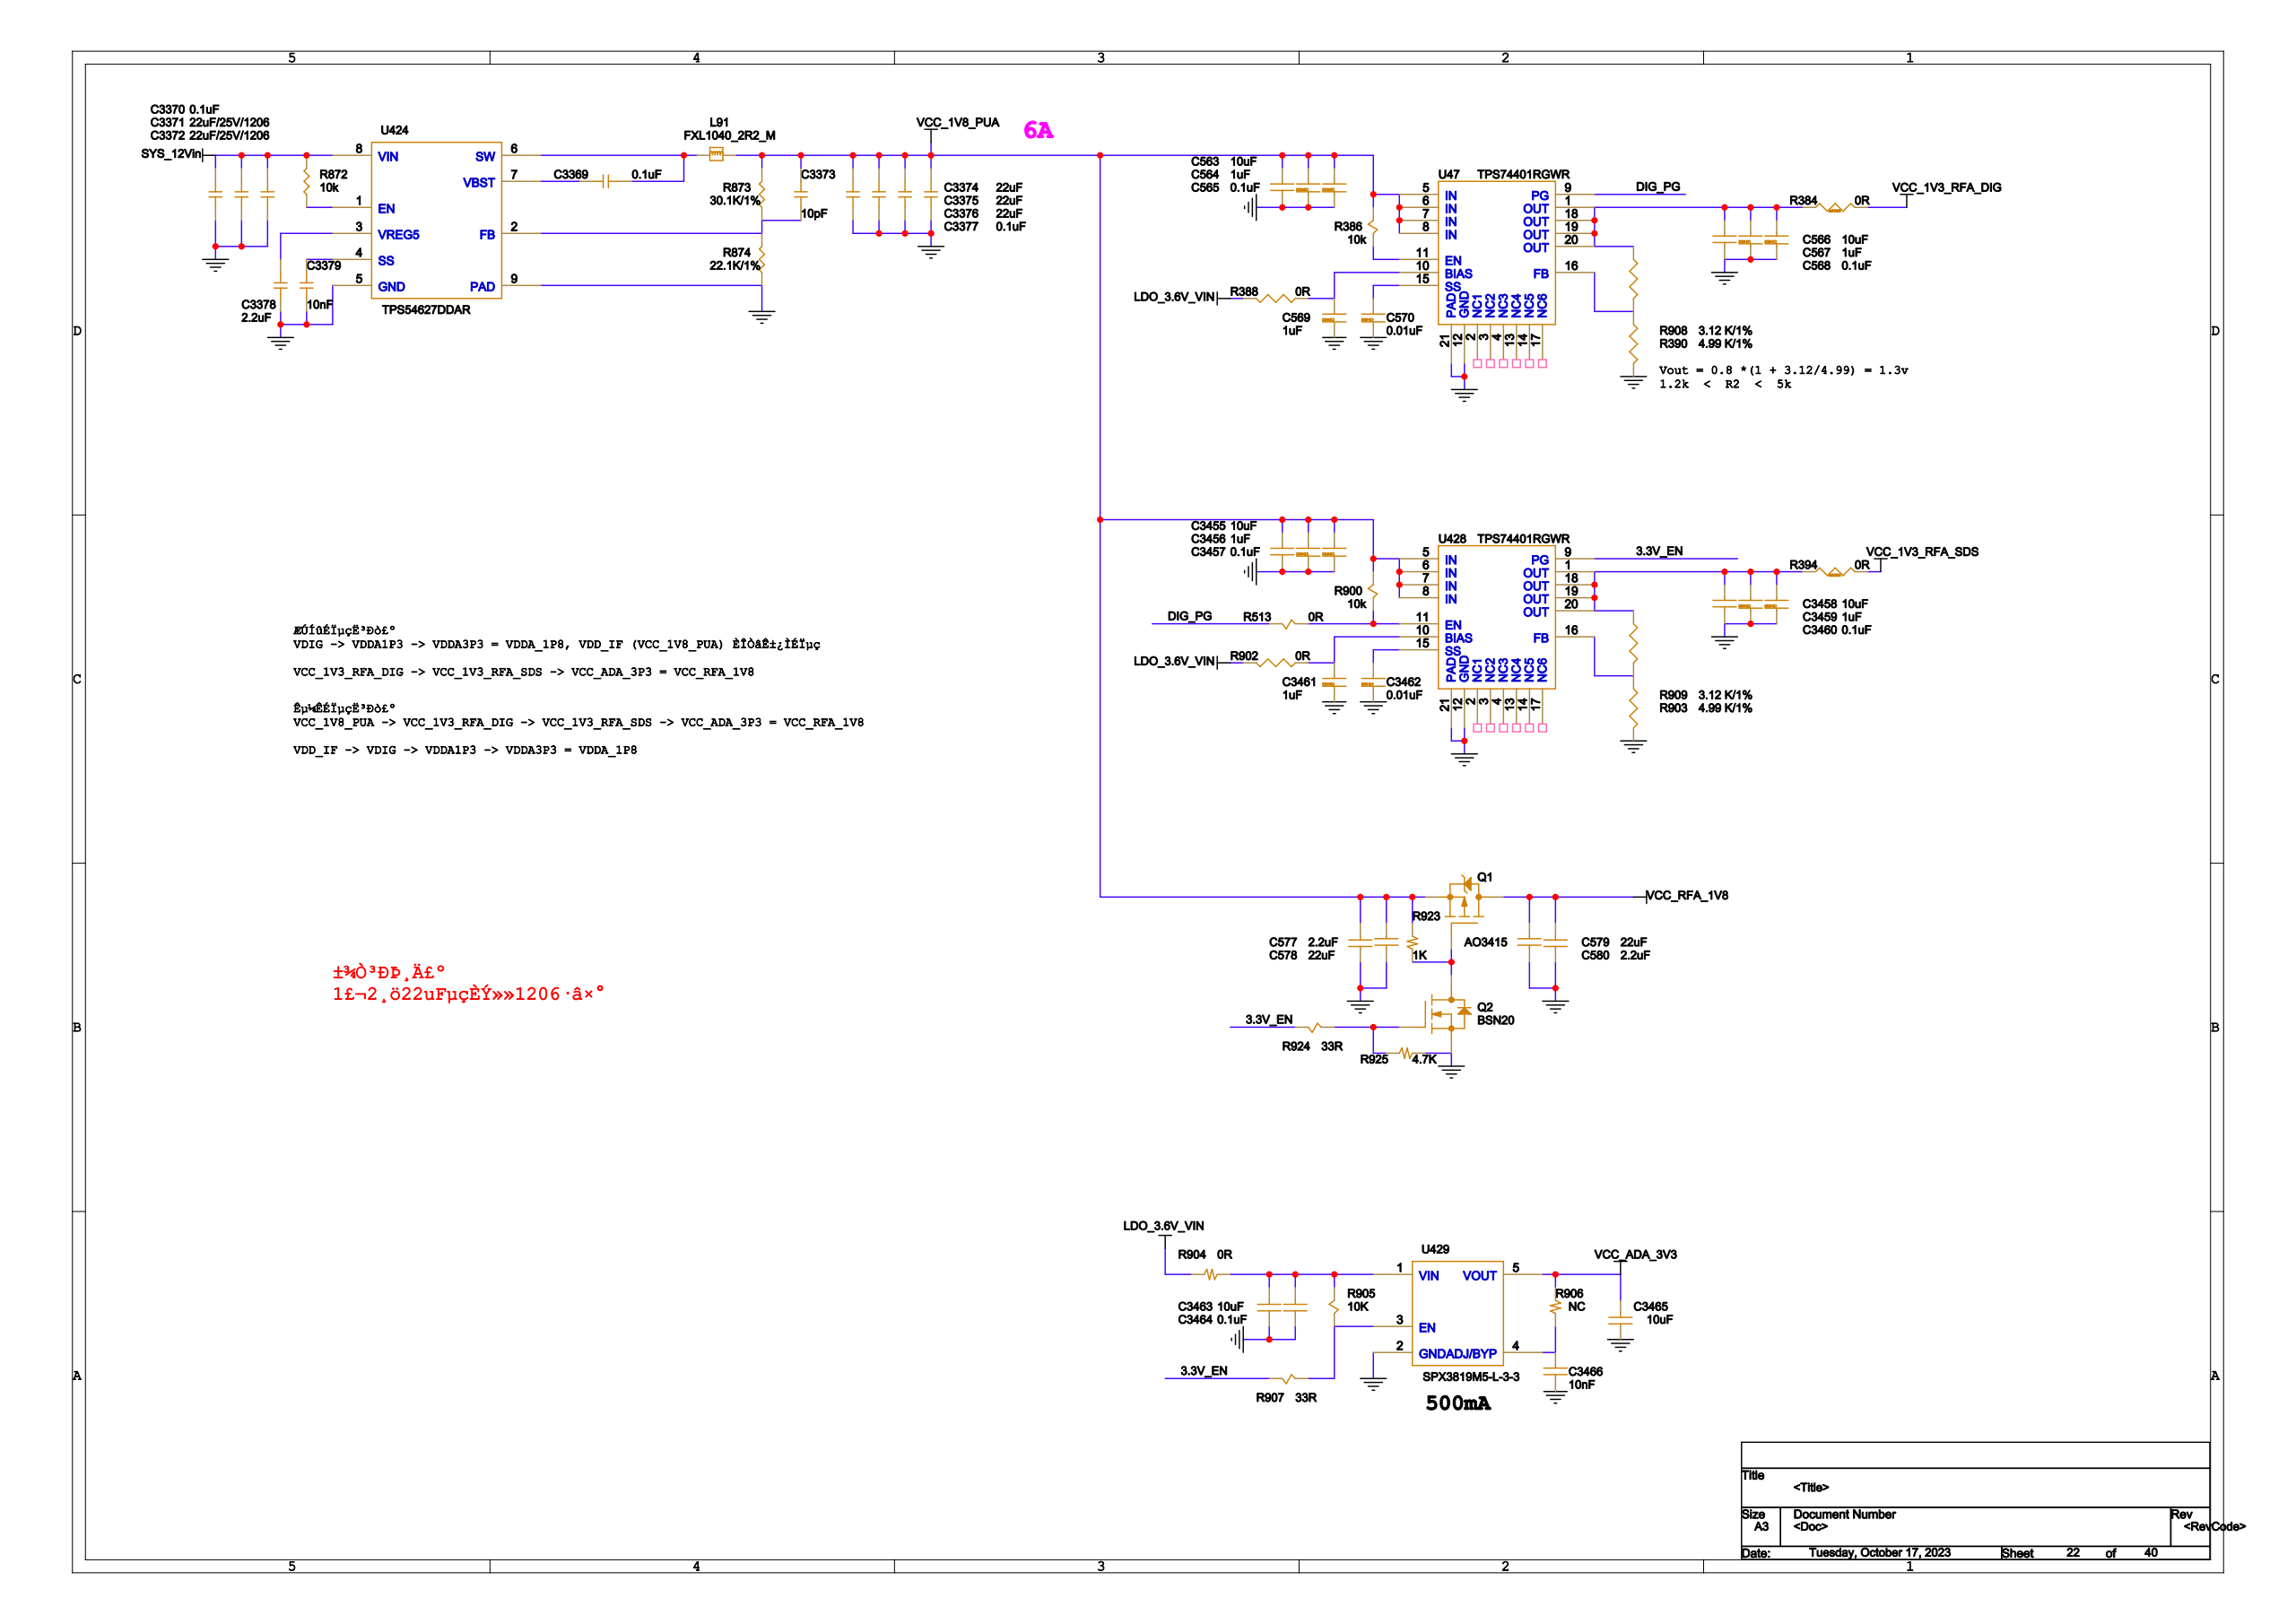Circuit board | Cadence Allegro | 1793 parts | 1223 nets | one sheet of the schematic
Parts on this sheet (reference | value | footprint):
C563 | 10uF | C0402
C564 | 1uF | C0402
C565 | 0.1uF | C0402
C566 | 10uF | C0402
C567 | 1uF | C0402
C568 | 0.1uF | C0402
C569 | 1uF | C0402
C570 | 0.01uF | C0402
C577 | 2.2uF | C0402
C578 | 22uF | C0603
C579 | 22uF | C0603
C580 | 2.2uF | C0402
C3369 | 0.1uF | C0402
C3370 | 0.1uF | C0402
C3371 | 22uF/25V/1206 | 1206
C3372 | 22uF/25V/1206 | 1206
C3373 | 10pF | C0402
C3374 | 22uF | C0603
C3375 | 22uF | C0603
C3376 | 22uF | C0603
C3377 | 0.1uF | C0402
C3378 | 2.2uF | C0402
C3379 | 10nF | C0402
C3455 | 10uF | C0402
C3456 | 1uF | C0402
C3457 | 0.1uF | C0402
C3458 | 10uF | C0402
C3459 | 1uF | C0402
C3460 | 0.1uF | C0402
C3461 | 1uF | C0402
C3462 | 0.01uF | C0402
C3463 | 10uF | C0402
C3464 | 0.1uF | C0402
C3465 | 10uF | C0402
C3466 | 10nF | C0402
L91 | FXL1040_2R2_M | SMD_11_5X10
Q1 | AO3415 | SOT23
Q2 | BSN20 | SOT23
R384 | 0R | R0805
R386 | 10K | R0402
R388 | 0R | R0402
R390 | 4.99 K/1% | R0402
R394 | 0R | R0805
R513 | 0R | R0402
R872 | 10k | R0402
R873 | 30.1K/1% | R0402
R874 | 22.1K/1% | R0402
R900 | 10K | R0402
R902 | 0R | R0402
R903 | 4.99 K/1% | R0402
R904 | 0R | R0402
R905 | 10K | R0402
R906 | NC | R0402
R907 | 33R | R0402
R908 | 3.12 K/1% | R0402
R909 | 3.12 K/1% | R0402
R923 | 1K | R0402
R924 | 33R | R0402
R925 | 4.7K | R0402
U47 | TPS74401RGWR | TPS74401RGWR_VQFN
U424 | TPS54627DDAR | POWER-SO8
U428 | TPS74401RGWR | TPS74401RGWR_VQFN
U429 | SPX3819M5-L-3-3 | SOT-23-5
Nets of these parts (net: part-pin ...):
GND: C563-2 C564-1 C565-1 C566-2 C567-1 C568-1 C569-1 C570-1 C577-1 C578-2 C579-2 C580-1 C3370-1 C3371-1 C3372-1 C3374-1 C3375-1 C3376-1 C3377-1 C3378-1 C3379-1 C3455-2 C3456-1 C3457-1 C3458-2 C3459-1 C3460-1 C3461-1 C3462-1 C3463-1 C3464-1 C3465-1 C3466-2 Q2-2 R390-2 R874-2 R903-2 R925-2 U47-12 U47-21 U424-5 U424-9 U428-12 U428-21 U429-2
SYS_12VIN: C3370-2 C3371-2 C3372-2 R872-1 U424-8
LDO_3.6V_VIN: R388-2 R902-2 R904-1
N16937054: R872-2 U424-1
VCC_1V3_RFA_SDS: R394-2
VCC_1V3_RFA_DIG: R384-2
VCC_RFA_1V8: C579-1 C580-2 Q1-3
VCC_1V8_PUA: C563-1 C564-2 C565-2 C577-2 C578-1 C3373-2 C3374-2 C3375-2 C3376-2 C3377-2 C3455-1 C3456-2 C3457-2 L91-2 Q1-2 R386-2 R873-1 R900-2 R923-1 U47-5 U47-6 U47-7 U47-8 U428-5 U428-6 U428-7 U428-8
N16937122: C3379-2 U424-4
N17089458: C3458-1 C3459-2 C3460-2 R394-1 R909-1 U428-1 U428-18 U428-19 U428-20
N985694: C566-1 C567-2 C568-2 R384-1 R908-1 U47-1 U47-18 U47-19 U47-20
N17091056: C3463-2 C3464-2 R904-2 R905-2 U429-1
VCC_ADA_3V3: C3465-2 R906-1 U429-5
N16937074: C3378-2 U424-3
N16936888: C3369-2 L91-1 U424-6
N16937062: C3373-1 R873-2 R874-1 U424-2
N16936978: C3369-1 U424-7
N17089524: C3461-2 R902-1 U428-10
N17089510: R513-1 R900-1 U428-11
N17089528: R903-1 R909-2 U428-16
3.3V_EN: R907-2 R924-2 U428-9
N17089552: C3462-2 U428-15
N15966415: C569-2 R388-1 U47-10
N985858: R386-1 U47-11
N985894: R390-1 R908-2 U47-16
DIG_PG: R513-2 U47-9
N985934: C570-2 U47-15
N17091131: C3466-1 R906-2 U429-4
N17164617: Q1-1 Q2-3 R923-2
N17165048: Q2-1 R924-1 R925-1
N17091127: R905-1 R907-1 U429-3